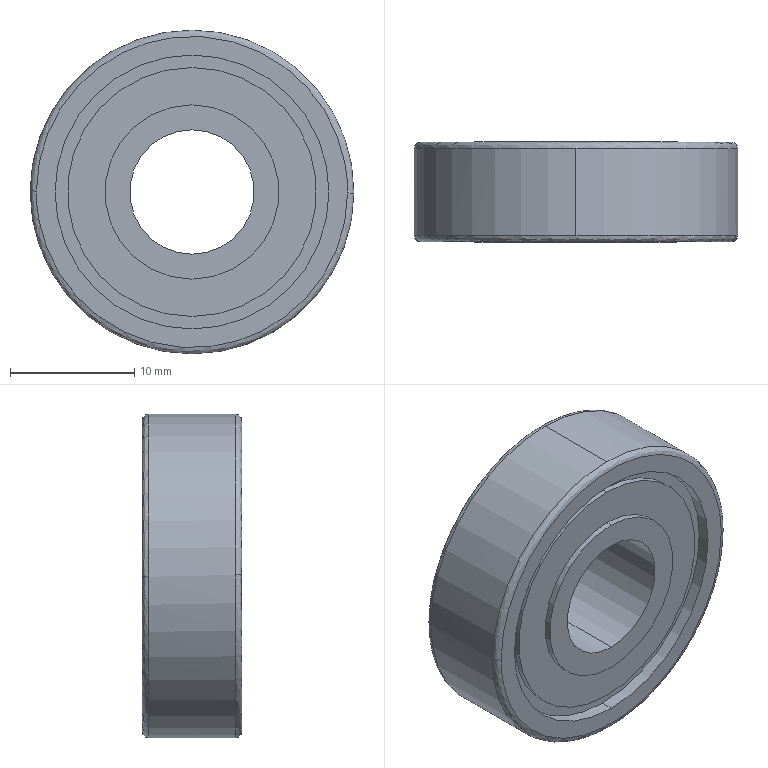Part | STEP file | 1 solid | 28 faces | box 26 x 8 x 26 mm | volume 3318 mm3 | cylinder 16 | plane 8 | spline 4 | commonest cylinder face diameters 14 x4 20 x4 22 x4 10 x2 26 x2